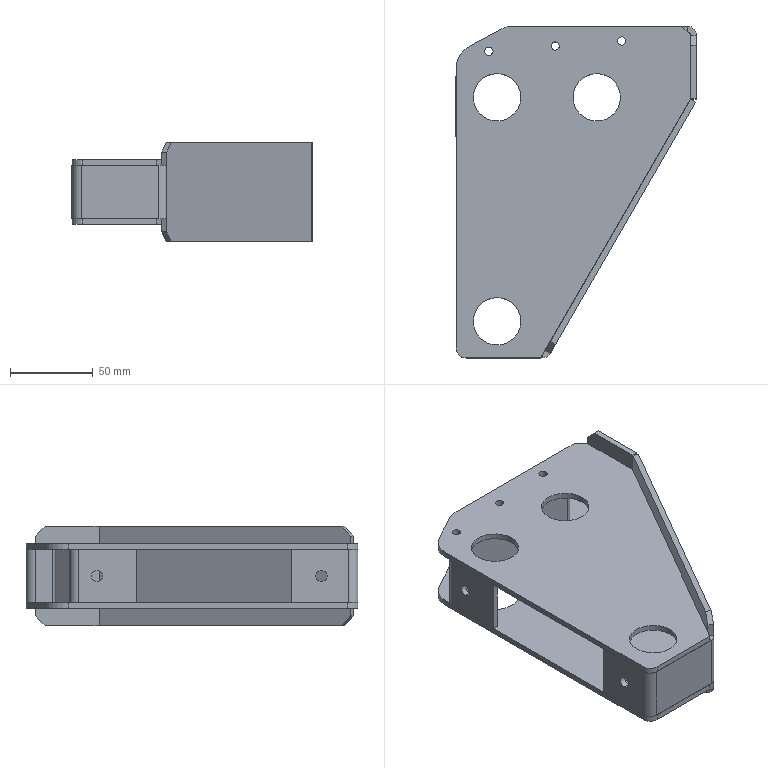Part | STEP file | ACTIVACION MECANICA UPPER RH SLIM V2.1_SLIM V3<Como mecanizada> | 4 solids | 120 faces | box 145 x 200 x 60 mm | volume 208719 mm3 | plane 74 | cylinder 46 | commonest cylinder face diameters 5 x12 28.6 x12 4 x6 11 x6 6.8 x4 30 x4